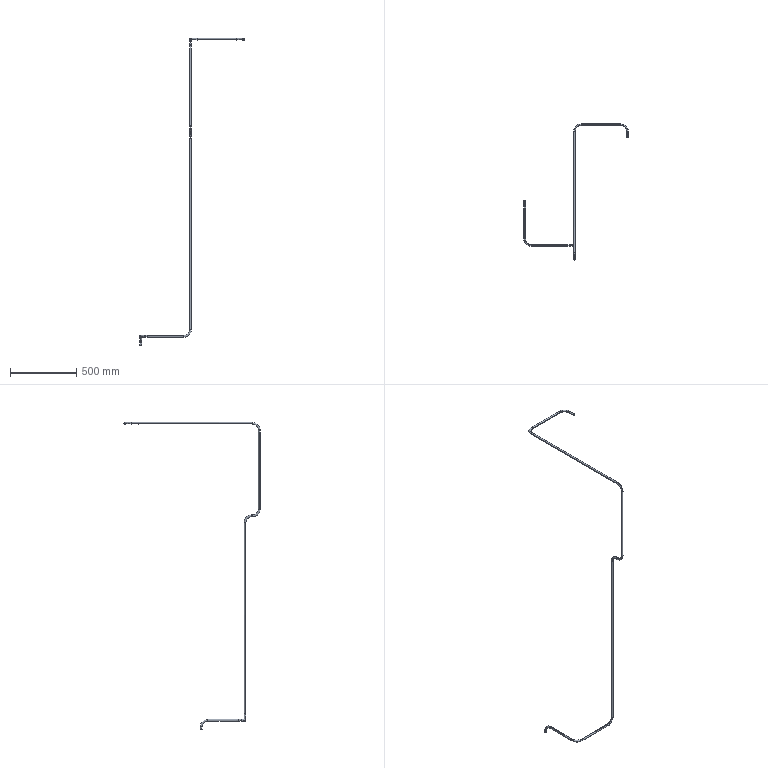Part | SolidWorks | features Sweep 5 | 1 solid | 70 faces | box 790.937 x 1030 x 2325 mm | volume 464272 mm3 | cylinder 36 | torus 32 | plane 2 | commonest cylinder face diameters 8 x18 14 x18